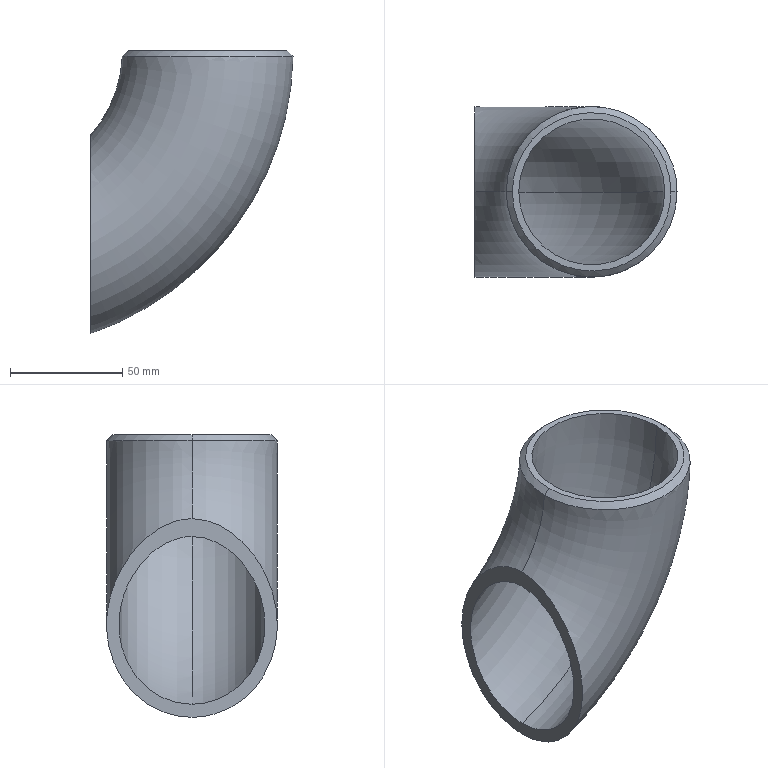Part | SolidWorks | features Chamfer 1, Revolution 1, Split 1 | 1 solid | 8 faces | box 89.972 x 76 x 125.857 mm | volume 125660 mm3 | torus 4 | spline 2 | plane 2
STEP:
#1=CARTESIAN_POINT('',(43.,0.,-37.417));
#2=VERTEX_POINT('',#1);
#3=CARTESIAN_POINT('',(43.,0.,-125.857));
#4=VERTEX_POINT('',#3);
#5=CARTESIAN_POINT('',(43.,0.,-37.417));
#6=CARTESIAN_POINT('',(43.,-2.709,-37.417));
#7=CARTESIAN_POINT('',(43.,-5.352,-37.856));
#8=CARTESIAN_POINT('',(43.,-9.232,-39.095));
#9=CARTESIAN_POINT('',(43.,-10.484,-39.596));
#10=CARTESIAN_POINT('',(43.,-12.905,-40.744));
#11=CARTESIAN_POINT('',(43.,-14.077,-41.391));
#12=CARTESIAN_POINT('',(43.,-15.785,-42.457));
#13=CARTESIAN_POINT('',(43.,-16.345,-42.829));
#14=CARTESIAN_POINT('',(43.,-17.45,-43.603));
#15=CARTESIAN_POINT('',(43.,-17.996,-44.006));
#16=CARTESIAN_POINT('',(43.,-19.594,-45.248));
#17=CARTESIAN_POINT('',(43.,-20.612,-46.122));
#18=CARTESIAN_POINT('',(43.,-23.541,-48.861));
#19=CARTESIAN_POINT('',(43.,-25.328,-50.845));
#20=CARTESIAN_POINT('',(43.,-27.377,-53.503));
#21=CARTESIAN_POINT('',(43.,-27.777,-54.043));
#22=CARTESIAN_POINT('',(43.,-28.559,-55.142));
#23=CARTESIAN_POINT('',(43.,-28.94,-55.7));
#24=CARTESIAN_POINT('',(43.,-30.047,-57.389));
#25=CARTESIAN_POINT('',(43.,-30.74,-58.538));
#26=CARTESIAN_POINT('',(43.,-32.684,-62.049));
#27=CARTESIAN_POINT('',(43.,-33.803,-64.476));
#28=CARTESIAN_POINT('',(43.,-34.976,-67.621));
#29=CARTESIAN_POINT('',(43.,-35.199,-68.256));
#30=CARTESIAN_POINT('',(43.,-35.622,-69.536));
#31=CARTESIAN_POINT('',(43.,-35.822,-70.182));
#32=CARTESIAN_POINT('',(43.,-36.381,-72.122));
#33=CARTESIAN_POINT('',(43.,-36.702,-73.421));
#34=CARTESIAN_POINT('',(43.,-37.509,-77.339));
#35=CARTESIAN_POINT('',(43.,-37.841,-79.978));
#36=CARTESIAN_POINT('',(43.,-38.013,-83.978));
#37=CARTESIAN_POINT('',(43.,-38.015,-85.318));
#38=CARTESIAN_POINT('',(43.,-37.932,-87.34));
#39=CARTESIAN_POINT('',(43.,-37.89,-88.016));
#40=CARTESIAN_POINT('',(43.,-37.776,-89.358));
#41=CARTESIAN_POINT('',(43.,-37.705,-90.025));
#42=CARTESIAN_POINT('',(43.,-37.277,-93.344));
#43=CARTESIAN_POINT('',(43.,-36.707,-95.942));
#44=CARTESIAN_POINT('',(43.,-35.496,-99.749));
#45=CARTESIAN_POINT('',(43.,-35.033,-101.003));
#46=CARTESIAN_POINT('',(43.,-34.243,-102.861));
#47=CARTESIAN_POINT('',(43.,-33.963,-103.477));
#48=CARTESIAN_POINT('',(43.,-33.374,-104.695));
#49=CARTESIAN_POINT('',(43.,-33.066,-105.295));
#50=CARTESIAN_POINT('',(43.,-31.456,-108.246));
#51=CARTESIAN_POINT('',(43.,-29.95,-110.458));
#52=CARTESIAN_POINT('',(43.,-27.786,-113.027));
#53=CARTESIAN_POINT('',(43.,-27.339,-113.531));
#54=CARTESIAN_POINT('',(43.,-26.415,-114.518));
#55=CARTESIAN_POINT('',(43.,-25.939,-115.001));
#56=CARTESIAN_POINT('',(43.,-24.483,-116.403));
#57=CARTESIAN_POINT('',(43.,-23.47,-117.28));
#58=CARTESIAN_POINT('',(43.,-21.36,-118.92));
#59=CARTESIAN_POINT('',(43.,-20.263,-119.684));
#60=CARTESIAN_POINT('',(43.,-18.553,-120.741));
#61=CARTESIAN_POINT('',(43.,-17.972,-121.079));
#62=CARTESIAN_POINT('',(43.,-16.788,-121.725));
#63=CARTESIAN_POINT('',(43.,-16.184,-122.034));
#64=CARTESIAN_POINT('',(43.,-13.137,-123.485));
#65=CARTESIAN_POINT('',(43.,-10.613,-124.361));
#66=CARTESIAN_POINT('',(43.,-7.351,-125.105));
#67=CARTESIAN_POINT('',(43.,-6.693,-125.236));
#68=CARTESIAN_POINT('',(43.,-5.366,-125.461));
#69=CARTESIAN_POINT('',(43.,-4.695,-125.556));
#70=CARTESIAN_POINT('',(43.,-2.678,-125.783));
#71=CARTESIAN_POINT('',(43.,-1.337,-125.857));
#72=CARTESIAN_POINT('',(43.,0.,-125.857));
#73=B_SPLINE_CURVE_WITH_KNOTS('',3,(#5,#6,#7,#8,#9,#10,#11,#12,#13,#14,#15,#16,#17,#18,#19,#20,#21,#22,#23,#24,#25,#26,#27,#28,#29,#30,#31,#32,#33,#34,#35,#36,#37,#38,#39,#40,#41,#42,#43,#44,#45,#46,#47,#48,#49,#50,#51,#52,#53,#54,#55,#56,#57,#58,#59,#60,#61,#62,#63,#64,#65,#66,#67,#68,#69,#70,#71,#72),.UNSPECIFIED.,.F.,.F.,(4,2,2,2,2,2,2,2,2,2,2,2,2,2,2,2,2,2,2,2,2,2,2,2,2,2,2,2,2,2,2,2,2,4),(0.1576,0.1656,0.1696,0.1736,0.1756,0.1776,0.1816,0.1896,0.1916,0.1936,0.1977,0.2057,0.2077,0.2097,0.2137,0.2217,0.2257,0.2277,0.2297,0.2377,0.2417,0.2437,0.2457,0.2538,0.2558,0.2578,0.2618,0.2658,0.2678,0.2698,0.2778,0.2798,0.2818,0.2858),.UNSPECIFIED.);
#74=EDGE_CURVE('',#2,#4,#73,.T.);
#75=ORIENTED_EDGE('',*,*,#74,.T.);
#76=CARTESIAN_POINT('',(132.972,0.,-2.722));
#77=VERTEX_POINT('',#76);
#78=CARTESIAN_POINT('',(0.,0.,0.));
#79=DIRECTION('',(0.,-1.,0.));
#80=DIRECTION('',(0.,0.,-1.));
#81=AXIS2_PLACEMENT_3D('',#78,#79,#80);
#82=CIRCLE('',#81,133.);
#83=EDGE_CURVE('',#4,#77,#82,.T.);
#84=ORIENTED_EDGE('',*,*,#83,.T.);
#85=CARTESIAN_POINT('',(56.943,-0.01359,-2.545));
#86=VERTEX_POINT('',#85);
#87=CARTESIAN_POINT('',(132.972,0.,-2.722));
#88=CARTESIAN_POINT('',(132.972,-2.665,-2.722));
#89=CARTESIAN_POINT('',(132.691,-5.307,-2.722));
#90=CARTESIAN_POINT('',(131.605,-10.435,-2.72));
#91=CARTESIAN_POINT('',(130.801,-12.92,-2.719));
#92=CARTESIAN_POINT('',(128.728,-17.638,-2.717));
#93=CARTESIAN_POINT('',(127.461,-19.87,-2.716));
#94=CARTESIAN_POINT('',(124.537,-24.005,-2.713));
#95=CARTESIAN_POINT('',(122.881,-25.907,-2.711));
#96=CARTESIAN_POINT('',(119.264,-29.325,-2.707));
#97=CARTESIAN_POINT('',(117.304,-30.84,-2.704));
#98=CARTESIAN_POINT('',(113.17,-33.446,-2.699));
#99=CARTESIAN_POINT('',(110.996,-34.537,-2.696));
#100=CARTESIAN_POINT('',(106.524,-36.279,-2.688));
#101=CARTESIAN_POINT('',(104.227,-36.929,-2.684));
#102=CARTESIAN_POINT('',(100.754,-37.575,-2.678));
#103=CARTESIAN_POINT('',(99.592,-37.735,-2.676));
#104=CARTESIAN_POINT('',(97.849,-37.895,-2.672));
#105=CARTESIAN_POINT('',(97.268,-37.934,-2.671));
#106=CARTESIAN_POINT('',(96.399,-37.974,-2.669));
#107=CARTESIAN_POINT('',(96.109,-37.984,-2.669));
#108=CARTESIAN_POINT('',(95.53,-37.997,-2.668));
#109=CARTESIAN_POINT('',(95.242,-38.,-2.667));
#110=CARTESIAN_POINT('',(92.627,-37.999,-2.662));
#111=CARTESIAN_POINT('',(90.221,-37.785,-2.657));
#112=CARTESIAN_POINT('',(86.56,-37.081,-2.648));
#113=CARTESIAN_POINT('',(85.331,-36.782,-2.645));
#114=CARTESIAN_POINT('',(83.487,-36.233,-2.641));
#115=CARTESIAN_POINT('',(82.872,-36.033,-2.639));
#116=CARTESIAN_POINT('',(81.951,-35.706,-2.636));
#117=CARTESIAN_POINT('',(81.49,-35.536,-2.635));
#118=CARTESIAN_POINT('',(80.954,-35.327,-2.634));
#119=CARTESIAN_POINT('',(80.687,-35.219,-2.633));
#120=CARTESIAN_POINT('',(80.553,-35.164,-2.633));
#121=CARTESIAN_POINT('',(80.496,-35.141,-2.633));
#122=CARTESIAN_POINT('',(80.457,-35.125,-2.632));
#123=CARTESIAN_POINT('',(80.437,-35.117,-2.632));
#124=CARTESIAN_POINT('',(78.122,-34.159,-2.626));
#125=CARTESIAN_POINT('',(75.919,-32.982,-2.618));
#126=CARTESIAN_POINT('',(72.818,-30.913,-2.607));
#127=CARTESIAN_POINT('',(71.818,-30.172,-2.604));
#128=CARTESIAN_POINT('',(70.377,-28.99,-2.599));
#129=CARTESIAN_POINT('',(69.906,-28.585,-2.598));
#130=CARTESIAN_POINT('',(69.215,-27.959,-2.596));
#131=CARTESIAN_POINT('',(68.873,-27.642,-2.595));
#132=CARTESIAN_POINT('',(68.481,-27.265,-2.594));
#133=CARTESIAN_POINT('',(68.287,-27.075,-2.594));
#134=CARTESIAN_POINT('',(68.19,-26.979,-2.593));
#135=CARTESIAN_POINT('',(68.142,-26.932,-2.593));
#136=CARTESIAN_POINT('',(68.122,-26.911,-2.593));
#137=CARTESIAN_POINT('',(68.108,-26.897,-2.593));
#138=CARTESIAN_POINT('',(68.102,-26.892,-2.593));
#139=CARTESIAN_POINT('',(66.006,-24.799,-2.589));
#140=CARTESIAN_POINT('',(64.246,-22.556,-2.58));
#141=CARTESIAN_POINT('',(61.346,-17.956,-2.565));
#142=CARTESIAN_POINT('',(60.206,-15.6,-2.558));
#143=CARTESIAN_POINT('',(58.468,-10.938,-2.549));
#144=CARTESIAN_POINT('',(57.869,-8.632,-2.546));
#145=CARTESIAN_POINT('',(57.297,-5.295,-2.545));
#146=CARTESIAN_POINT('',(57.161,-4.203,-2.545));
#147=CARTESIAN_POINT('',(57.029,-2.602,-2.545));
#148=CARTESIAN_POINT('',(56.996,-2.075,-2.545));
#149=CARTESIAN_POINT('',(56.964,-1.294,-2.545));
#150=CARTESIAN_POINT('',(56.952,-0.9063,-2.545));
#151=CARTESIAN_POINT('',(56.946,-0.4584,-2.545));
#152=CARTESIAN_POINT('',(56.944,-0.2356,-2.545));
#153=CARTESIAN_POINT('',(56.943,-0.1245,-2.545));
#154=CARTESIAN_POINT('',(56.943,-0.06902,-2.545));
#155=CARTESIAN_POINT('',(56.943,-0.04526,-2.545));
#156=CARTESIAN_POINT('',(56.943,-0.02942,-2.545));
#157=CARTESIAN_POINT('',(56.943,-0.02269,-2.545));
#158=CARTESIAN_POINT('',(56.943,-0.01359,-2.545));
#159=B_SPLINE_CURVE_WITH_KNOTS('',3,(#87,#88,#89,#90,#91,#92,#93,#94,#95,#96,#97,#98,#99,#100,#101,#102,#103,#104,#105,#106,#107,#108,#109,#110,#111,#112,#113,#114,#115,#116,#117,#118,#119,#120,#121,#122,#123,#124,#125,#126,#127,#128,#129,#130,#131,#132,#133,#134,#135,#136,#137,#138,#139,#140,#141,#142,#143,#144,#145,#146,#147,#148,#149,#150,#151,#152,#153,#154,#155,#156,#157,#158),.UNSPECIFIED.,.F.,.F.,(4,2,2,2,2,2,2,2,2,2,2,2,2,2,2,1,1,1,1,2,2,2,2,2,1,1,1,1,1,2,2,2,2,2,2,2,1,1,1,1,1,2,4),(0.,0.03125,0.0625,0.09375,0.125,0.1563,0.1875,0.2188,0.2344,0.2422,0.2461,0.25,0.2813,0.2969,0.3047,0.3086,0.3105,0.3115,0.312,0.3123,0.3125,0.3438,0.3594,0.3672,0.3711,0.373,0.374,0.3745,0.3748,0.3749,0.375,0.4063,0.4375,0.4688,0.4844,0.4922,0.4961,0.498,0.499,0.4995,0.4998,0.4999,0.5),.UNSPECIFIED.);
#160=EDGE_CURVE('',#77,#86,#159,.T.);
#161=ORIENTED_EDGE('',*,*,#160,.T.);
#162=CARTESIAN_POINT('',(0.,0.,0.));
#163=DIRECTION('',(0.,-1.,0.));
#164=DIRECTION('',(0.,0.,-1.));
#165=AXIS2_PLACEMENT_3D('',#162,#163,#164);
#166=CIRCLE('',#165,57.);
#167=EDGE_CURVE('',#2,#86,#166,.T.);
#168=ORIENTED_EDGE('',*,*,#167,.F.);
#169=EDGE_LOOP('',(#75,#84,#161,#168));
#170=FACE_OUTER_BOUND('',#169,.T.);
#171=CARTESIAN_POINT('',(0.,0.,0.));
#172=DIRECTION('',(0.,-1.,0.));
#173=DIRECTION('',(0.,0.,-1.));
#174=AXIS2_PLACEMENT_3D('',#171,#172,#173);
#175=TOROIDAL_SURFACE('',#174,95.,38.);
#176=ADVANCED_FACE('',(#170),#175,.T.);
#177=CARTESIAN_POINT('',(59.663,-0.01262,0.));
#178=VERTEX_POINT('',#177);
#179=CARTESIAN_POINT('',(130.25,0.,0.));
#180=VERTEX_POINT('',#179);
#181=CARTESIAN_POINT('',(59.663,-0.01262,0.));
#182=CARTESIAN_POINT('',(59.666,-2.359,0.));
#183=CARTESIAN_POINT('',(60.005,-5.807,0.));
#184=CARTESIAN_POINT('',(60.987,-9.705,0.));
#185=CARTESIAN_POINT('',(61.533,-11.349,0.));
#186=CARTESIAN_POINT('',(61.926,-12.44,0.));
#187=CARTESIAN_POINT('',(62.135,-12.98,0.));
#188=CARTESIAN_POINT('',(63.259,-15.684,0.));
#189=CARTESIAN_POINT('',(64.89,-18.736,0.));
#190=CARTESIAN_POINT('',(67.288,-21.959,0.));
#191=CARTESIAN_POINT('',(68.422,-23.268,0.));
#192=CARTESIAN_POINT('',(69.202,-24.125,0.));
#193=CARTESIAN_POINT('',(69.603,-24.544,0.));
#194=CARTESIAN_POINT('',(73.331,-28.262,0.));
#195=CARTESIAN_POINT('',(77.146,-30.808,0.));
#196=CARTESIAN_POINT('',(83.617,-33.486,0.));
#197=CARTESIAN_POINT('',(86.922,-34.491,0.));
#198=CARTESIAN_POINT('',(90.897,-35.079,0.));
#199=CARTESIAN_POINT('',(92.627,-35.206,0.));
#200=CARTESIAN_POINT('',(93.785,-35.262,0.));
#201=CARTESIAN_POINT('',(94.369,-35.277,0.));
#202=CARTESIAN_POINT('',(97.287,-35.279,0.));
#203=CARTESIAN_POINT('',(100.725,-34.946,0.));
#204=CARTESIAN_POINT('',(104.068,-34.108,0.));
#205=CARTESIAN_POINT('',(106.276,-33.437,0.));
#206=CARTESIAN_POINT('',(107.371,-33.045,0.));
#207=CARTESIAN_POINT('',(112.775,-30.812,0.));
#208=CARTESIAN_POINT('',(116.594,-28.263,0.));
#209=CARTESIAN_POINT('',(121.565,-23.297,0.));
#210=CARTESIAN_POINT('',(123.764,-20.624,0.));
#211=CARTESIAN_POINT('',(125.536,-17.666,0.));
#212=CARTESIAN_POINT('',(126.621,-15.63,0.));
#213=CARTESIAN_POINT('',(127.116,-14.582,0.));
#214=CARTESIAN_POINT('',(129.357,-9.17,0.));
#215=CARTESIAN_POINT('',(130.252,-4.67,0.));
#216=CARTESIAN_POINT('',(130.25,0.,0.));
#217=B_SPLINE_CURVE_WITH_KNOTS('',3,(#181,#182,#183,#184,#185,#186,#187,#188,#189,#190,#191,#192,#193,#194,#195,#196,#197,#198,#199,#200,#201,#202,#203,#204,#205,#206,#207,#208,#209,#210,#211,#212,#213,#214,#215,#216),.UNSPECIFIED.,.F.,.F.,(4,1,1,2,2,1,1,2,2,2,1,1,2,2,1,2,2,2,1,2,2,4),(0.5,0.5312,0.5469,0.5547,0.5625,0.5938,0.6094,0.6172,0.625,0.6875,0.7187,0.7344,0.7422,0.75,0.7812,0.7969,0.8125,0.875,0.9062,0.9219,0.9375,1.),.UNSPECIFIED.);
#218=EDGE_CURVE('',#178,#180,#217,.T.);
#219=ORIENTED_EDGE('',*,*,#218,.F.);
#220=CARTESIAN_POINT('',(59.663,-0.01262,0.));
#221=CARTESIAN_POINT('',(56.943,-0.01359,-2.545));
#222=B_SPLINE_CURVE_WITH_KNOTS('',1,(#220,#221),.UNSPECIFIED.,.F.,.F.,(2,2),(0.,1.),.UNSPECIFIED.);
#223=EDGE_CURVE('',#178,#86,#222,.T.);
#224=ORIENTED_EDGE('',*,*,#223,.T.);
#225=ORIENTED_EDGE('',*,*,#160,.F.);
#226=CARTESIAN_POINT('',(130.25,0.,0.));
#227=CARTESIAN_POINT('',(132.972,0.,-2.722));
#228=B_SPLINE_CURVE_WITH_KNOTS('',1,(#226,#227),.UNSPECIFIED.,.F.,.F.,(2,2),(0.,1.),.UNSPECIFIED.);
#229=EDGE_CURVE('',#180,#77,#228,.T.);
#230=ORIENTED_EDGE('',*,*,#229,.F.);
#231=EDGE_LOOP('',(#219,#224,#225,#230));
#232=FACE_OUTER_BOUND('',#231,.T.);
#233=CARTESIAN_POINT('',(130.25,0.,0.));
#234=CARTESIAN_POINT('',(130.249,2.299,0.));
#235=CARTESIAN_POINT('',(130.028,4.585,0.));
#236=CARTESIAN_POINT('',(129.123,9.145,0.));
#237=CARTESIAN_POINT('',(128.445,11.372,0.));
#238=CARTESIAN_POINT('',(126.689,15.614,0.));
#239=CARTESIAN_POINT('',(125.599,17.66,0.));
#240=CARTESIAN_POINT('',(123.011,21.532,0.));
#241=CARTESIAN_POINT('',(121.549,23.308,0.));
#242=CARTESIAN_POINT('',(118.305,26.558,0.));
#243=CARTESIAN_POINT('',(116.488,28.051,0.));
#244=CARTESIAN_POINT('',(112.647,30.614,0.));
#245=CARTESIAN_POINT('',(110.623,31.697,0.));
#246=CARTESIAN_POINT('',(106.353,33.47,0.));
#247=CARTESIAN_POINT('',(104.106,34.151,0.));
#248=CARTESIAN_POINT('',(99.603,35.045,0.));
#249=CARTESIAN_POINT('',(97.312,35.276,0.));
#250=CARTESIAN_POINT('',(92.651,35.279,0.));
#251=CARTESIAN_POINT('',(90.35,35.049,0.));
#252=CARTESIAN_POINT('',(85.847,34.158,0.));
#253=CARTESIAN_POINT('',(83.612,33.484,0.));
#254=CARTESIAN_POINT('',(79.323,31.709,0.));
#255=CARTESIAN_POINT('',(77.298,30.626,0.));
#256=CARTESIAN_POINT('',(73.467,28.076,0.));
#257=CARTESIAN_POINT('',(71.644,26.583,0.));
#258=CARTESIAN_POINT('',(68.39,23.331,0.));
#259=CARTESIAN_POINT('',(66.928,21.56,0.));
#260=CARTESIAN_POINT('',(64.342,17.702,0.));
#261=CARTESIAN_POINT('',(63.242,15.645,0.));
#262=CARTESIAN_POINT('',(60.602,9.288,0.));
#263=CARTESIAN_POINT('',(59.658,4.638,0.));
#264=CARTESIAN_POINT('',(59.666,-2.338,0.));
#265=CARTESIAN_POINT('',(59.895,-4.639,0.));
#266=CARTESIAN_POINT('',(60.791,-9.141,0.));
#267=CARTESIAN_POINT('',(61.471,-11.382,0.));
#268=CARTESIAN_POINT('',(63.249,-15.66,0.));
#269=CARTESIAN_POINT('',(64.334,-17.683,0.));
#270=CARTESIAN_POINT('',(66.895,-21.516,0.));
#271=CARTESIAN_POINT('',(68.39,-23.335,0.));
#272=CARTESIAN_POINT('',(71.644,-26.58,0.));
#273=CARTESIAN_POINT('',(73.419,-28.04,0.));
#274=CARTESIAN_POINT('',(77.288,-30.624,0.));
#275=CARTESIAN_POINT('',(79.339,-31.716,0.));
#276=CARTESIAN_POINT('',(83.581,-33.471,0.));
#277=CARTESIAN_POINT('',(85.802,-34.148,0.));
#278=CARTESIAN_POINT('',(90.368,-35.054,0.));
#279=CARTESIAN_POINT('',(92.656,-35.276,0.));
#280=CARTESIAN_POINT('',(97.25,-35.279,0.));
#281=CARTESIAN_POINT('',(99.592,-35.049,0.));
#282=CARTESIAN_POINT('',(104.115,-34.147,0.));
#283=CARTESIAN_POINT('',(106.313,-33.482,0.));
#284=CARTESIAN_POINT('',(110.591,-31.715,0.));
#285=CARTESIAN_POINT('',(112.658,-30.609,0.));
#286=CARTESIAN_POINT('',(116.474,-28.058,0.));
#287=CARTESIAN_POINT('',(118.259,-26.6,0.));
#288=CARTESIAN_POINT('',(121.557,-23.305,0.));
#289=CARTESIAN_POINT('',(123.02,-21.517,0.));
#290=CARTESIAN_POINT('',(125.573,-17.702,0.));
#291=CARTESIAN_POINT('',(126.677,-15.642,0.));
#292=CARTESIAN_POINT('',(128.452,-11.357,0.));
#293=CARTESIAN_POINT('',(129.117,-9.159,0.));
#294=CARTESIAN_POINT('',(130.02,-4.643,0.));
#295=CARTESIAN_POINT('',(130.251,-2.299,0.));
#296=CARTESIAN_POINT('',(130.25,0.,0.));
#297=CARTESIAN_POINT('',(132.972,0.,-2.722));
#298=CARTESIAN_POINT('',(132.971,2.476,-2.722));
#299=CARTESIAN_POINT('',(132.733,4.939,-2.722));
#300=CARTESIAN_POINT('',(131.758,9.851,-2.721));
#301=CARTESIAN_POINT('',(131.028,12.25,-2.72));
#302=CARTESIAN_POINT('',(129.136,16.819,-2.718));
#303=CARTESIAN_POINT('',(127.963,19.023,-2.717));
#304=CARTESIAN_POINT('',(125.175,23.194,-2.713));
#305=CARTESIAN_POINT('',(123.6,25.107,-2.711));
#306=CARTESIAN_POINT('',(120.105,28.608,-2.707));
#307=CARTESIAN_POINT('',(118.148,30.216,-2.704));
#308=CARTESIAN_POINT('',(114.011,32.977,-2.699));
#309=CARTESIAN_POINT('',(111.831,34.143,-2.696));
#310=CARTESIAN_POINT('',(107.231,36.053,-2.689));
#311=CARTESIAN_POINT('',(104.811,36.787,-2.685));
#312=CARTESIAN_POINT('',(99.961,37.75,-2.676));
#313=CARTESIAN_POINT('',(97.493,37.999,-2.671));
#314=CARTESIAN_POINT('',(92.473,38.001,-2.661));
#315=CARTESIAN_POINT('',(89.994,37.754,-2.656));
#316=CARTESIAN_POINT('',(85.144,36.794,-2.645));
#317=CARTESIAN_POINT('',(82.737,36.068,-2.639));
#318=CARTESIAN_POINT('',(78.117,34.156,-2.626));
#319=CARTESIAN_POINT('',(75.936,32.99,-2.62));
#320=CARTESIAN_POINT('',(71.81,30.243,-2.606));
#321=CARTESIAN_POINT('',(69.846,28.635,-2.6));
#322=CARTESIAN_POINT('',(66.341,25.132,-2.587));
#323=CARTESIAN_POINT('',(64.768,23.224,-2.58));
#324=CARTESIAN_POINT('',(61.982,19.069,-2.569));
#325=CARTESIAN_POINT('',(60.797,16.852,-2.563));
#326=CARTESIAN_POINT('',(57.954,10.005,-2.55));
#327=CARTESIAN_POINT('',(56.938,4.996,-2.545));
#328=CARTESIAN_POINT('',(56.946,-2.518,-2.545));
#329=CARTESIAN_POINT('',(57.193,-4.997,-2.546));
#330=CARTESIAN_POINT('',(58.158,-9.847,-2.551));
#331=CARTESIAN_POINT('',(58.89,-12.261,-2.555));
#332=CARTESIAN_POINT('',(60.805,-16.869,-2.563));
#333=CARTESIAN_POINT('',(61.973,-19.048,-2.569));
#334=CARTESIAN_POINT('',(64.731,-23.177,-2.58));
#335=CARTESIAN_POINT('',(66.342,-25.136,-2.587));
#336=CARTESIAN_POINT('',(69.846,-28.631,-2.6));
#337=CARTESIAN_POINT('',(71.758,-30.204,-2.606));
#338=CARTESIAN_POINT('',(75.925,-32.987,-2.62));
#339=CARTESIAN_POINT('',(78.135,-34.164,-2.626));
#340=CARTESIAN_POINT('',(82.703,-36.055,-2.639));
#341=CARTESIAN_POINT('',(85.096,-36.783,-2.645));
#342=CARTESIAN_POINT('',(90.013,-37.76,-2.656));
#343=CARTESIAN_POINT('',(92.478,-37.998,-2.661));
#344=CARTESIAN_POINT('',(97.426,-38.002,-2.671));
#345=CARTESIAN_POINT('',(99.949,-37.754,-2.676));
#346=CARTESIAN_POINT('',(104.821,-36.783,-2.685));
#347=CARTESIAN_POINT('',(107.188,-36.066,-2.688));
#348=CARTESIAN_POINT('',(111.796,-34.162,-2.696));
#349=CARTESIAN_POINT('',(114.023,-32.971,-2.699));
#350=CARTESIAN_POINT('',(118.133,-30.223,-2.704));
#351=CARTESIAN_POINT('',(120.056,-28.653,-2.707));
#352=CARTESIAN_POINT('',(123.608,-25.103,-2.711));
#353=CARTESIAN_POINT('',(125.184,-23.178,-2.713));
#354=CARTESIAN_POINT('',(127.934,-19.068,-2.717));
#355=CARTESIAN_POINT('',(129.124,-16.849,-2.718));
#356=CARTESIAN_POINT('',(131.035,-12.233,-2.72));
#357=CARTESIAN_POINT('',(131.751,-9.866,-2.721));
#358=CARTESIAN_POINT('',(132.724,-5.002,-2.722));
#359=CARTESIAN_POINT('',(132.973,-2.476,-2.722));
#360=CARTESIAN_POINT('',(132.972,0.,-2.722));
#361=B_SPLINE_SURFACE_WITH_KNOTS('',1,3,((#233,#234,#235,#236,#237,#238,#239,#240,#241,#242,#243,#244,#245,#246,#247,#248,#249,#250,#251,#252,#253,#254,#255,#256,#257,#258,#259,#260,#261,#262,#263,#264,#265,#266,#267,#268,#269,#270,#271,#272,#273,#274,#275,#276,#277,#278,#279,#280,#281,#282,#283,#284,#285,#286,#287,#288,#289,#290,#291,#292,#293,#294,#295,#296),(#297,#298,#299,#300,#301,#302,#303,#304,#305,#306,#307,#308,#309,#310,#311,#312,#313,#314,#315,#316,#317,#318,#319,#320,#321,#322,#323,#324,#325,#326,#327,#328,#329,#330,#331,#332,#333,#334,#335,#336,#337,#338,#339,#340,#341,#342,#343,#344,#345,#346,#347,#348,#349,#350,#351,#352,#353,#354,#355,#356,#357,#358,#359,#360)),.UNSPECIFIED.,.F.,.T.,.F.,(2,2),(4,2,2,2,2,2,2,2,2,2,2,2,2,2,2,2,2,2,2,2,2,2,2,2,2,2,2,2,2,2,2,4),(0.,1.),(0.00369,0.01058,0.01748,0.02437,0.03127,0.03816,0.04505,0.05195,0.05884,0.06574,0.07263,0.07952,0.08642,0.09331,0.1002,0.114,0.1209,0.1278,0.1347,0.1416,0.1485,0.1554,0.1623,0.1691,0.176,0.1829,0.1898,0.1967,0.2036,0.2105,0.2174,0.2243),.UNSPECIFIED.);
#362=ADVANCED_FACE('',(#232),#361,.T.);
#363=CARTESIAN_POINT('',(43.,0.,-120.03));
#364=VERTEX_POINT('',#363);
#365=CARTESIAN_POINT('',(43.,0.,-45.357));
#366=VERTEX_POINT('',#365);
#367=CARTESIAN_POINT('',(43.,0.,-120.03));
#368=CARTESIAN_POINT('',(43.,1.143,-120.03));
#369=CARTESIAN_POINT('',(43.,2.299,-119.965));
#370=CARTESIAN_POINT('',(43.,4.57,-119.709));
#371=CARTESIAN_POINT('',(43.,5.692,-119.518));
#372=CARTESIAN_POINT('',(43.,7.907,-119.014));
#373=CARTESIAN_POINT('',(43.,9.,-118.701));
#374=CARTESIAN_POINT('',(43.,11.159,-117.952));
#375=CARTESIAN_POINT('',(43.,12.23,-117.512));
#376=CARTESIAN_POINT('',(43.,15.327,-116.038));
#377=CARTESIAN_POINT('',(43.,17.26,-114.843));
#378=CARTESIAN_POINT('',(43.,19.97,-112.744));
#379=CARTESIAN_POINT('',(43.,20.845,-111.988));
#380=CARTESIAN_POINT('',(43.,22.496,-110.404));
#381=CARTESIAN_POINT('',(43.,23.275,-109.574));
#382=CARTESIAN_POINT('',(43.,24.746,-107.841));
#383=CARTESIAN_POINT('',(43.,25.437,-106.937));
#384=CARTESIAN_POINT('',(43.,26.408,-105.527));
#385=CARTESIAN_POINT('',(43.,26.721,-105.048));
#386=CARTESIAN_POINT('',(43.,27.324,-104.072));
#387=CARTESIAN_POINT('',(43.,27.615,-103.575));
#388=CARTESIAN_POINT('',(43.,28.999,-101.067));
#389=CARTESIAN_POINT('',(43.,29.899,-98.979));
#390=CARTESIAN_POINT('',(43.,30.959,-95.732));
#391=CARTESIAN_POINT('',(43.,31.264,-94.63));
#392=CARTESIAN_POINT('',(43.,31.776,-92.388));
#393=CARTESIAN_POINT('',(43.,31.979,-91.263));
#394=CARTESIAN_POINT('',(43.,32.442,-87.879));
#395=CARTESIAN_POINT('',(43.,32.554,-85.609));
#396=CARTESIAN_POINT('',(43.,32.438,-82.185));
#397=CARTESIAN_POINT('',(43.,32.351,-81.036));
#398=CARTESIAN_POINT('',(43.,32.087,-78.764));
#399=CARTESIAN_POINT('',(43.,31.909,-77.639));
#400=CARTESIAN_POINT('',(43.,31.245,-74.296));
#401=CARTESIAN_POINT('',(43.,30.628,-72.11));
#402=CARTESIAN_POINT('',(43.,29.446,-68.894));
#403=CARTESIAN_POINT('',(43.,29.007,-67.829));
#404=CARTESIAN_POINT('',(43.,28.054,-65.752));
#405=CARTESIAN_POINT('',(43.,27.54,-64.738));
#406=CARTESIAN_POINT('',(43.,25.887,-61.764));
#407=CARTESIAN_POINT('',(43.,24.636,-59.875));
#408=CARTESIAN_POINT('',(43.,22.876,-57.637));
#409=CARTESIAN_POINT('',(43.,22.514,-57.196));
#410=CARTESIAN_POINT('',(43.,21.77,-56.326));
#411=CARTESIAN_POINT('',(43.,21.386,-55.897));
#412=CARTESIAN_POINT('',(43.,20.212,-54.64));
#413=CARTESIAN_POINT('',(43.,19.397,-53.841));
#414=CARTESIAN_POINT('',(43.,16.854,-51.566));
#415=CARTESIAN_POINT('',(43.,15.028,-50.21));
#416=CARTESIAN_POINT('',(43.,12.544,-48.763));
#417=CARTESIAN_POINT('',(43.,12.038,-48.486));
#418=CARTESIAN_POINT('',(43.,11.017,-47.967));
#419=CARTESIAN_POINT('',(43.,10.5,-47.724));
#420=CARTESIAN_POINT('',(43.,8.933,-47.042));
#421=CARTESIAN_POINT('',(43.,7.863,-46.652));
#422=CARTESIAN_POINT('',(43.,6.219,-46.174));
#423=CARTESIAN_POINT('',(43.,5.665,-46.033));
#424=CARTESIAN_POINT('',(43.,4.541,-45.789));
#425=CARTESIAN_POINT('',(43.,3.972,-45.685));
#426=CARTESIAN_POINT('',(43.,2.27,-45.439));
#427=CARTESIAN_POINT('',(43.,1.135,-45.357));
#428=CARTESIAN_POINT('',(43.,0.,-45.357));
#429=B_SPLINE_CURVE_WITH_KNOTS('',3,(#367,#368,#369,#370,#371,#372,#373,#374,#375,#376,#377,#378,#379,#380,#381,#382,#383,#384,#385,#386,#387,#388,#389,#390,#391,#392,#393,#394,#395,#396,#397,#398,#399,#400,#401,#402,#403,#404,#405,#406,#407,#408,#409,#410,#411,#412,#413,#414,#415,#416,#417,#418,#419,#420,#421,#422,#423,#424,#425,#426,#427,#428),.UNSPECIFIED.,.F.,.F.,(4,2,2,2,2,2,2,2,2,2,2,2,2,2,2,2,2,2,2,2,2,2,2,2,2,2,2,2,2,2,4),(0.01925,0.02266,0.02607,0.02948,0.03288,0.0397,0.0431,0.04651,0.04992,0.05162,0.05333,0.06014,0.06355,0.06695,0.07377,0.07718,0.08058,0.0874,0.09081,0.09421,0.101,0.1027,0.1044,0.1078,0.1147,0.1164,0.1181,0.1215,0.1232,0.1249,0.1283),.UNSPECIFIED.);
#430=EDGE_CURVE('',#364,#366,#429,.T.);
#431=ORIENTED_EDGE('',*,*,#430,.F.);
#432=CARTESIAN_POINT('',(127.5,0.,0.));
#433=VERTEX_POINT('',#432);
#434=CARTESIAN_POINT('',(0.,0.,0.));
#435=DIRECTION('',(0.,-1.,0.));
#436=DIRECTION('',(0.,0.,-1.));
#437=AXIS2_PLACEMENT_3D('',#434,#435,#436);
#438=CIRCLE('',#437,127.5);
#439=EDGE_CURVE('',#364,#433,#438,.T.);
#440=ORIENTED_EDGE('',*,*,#439,.T.);
#441=CARTESIAN_POINT('',(62.5,0.,0.));
#442=VERTEX_POINT('',#441);
#443=CARTESIAN_POINT('',(95.,0.,0.));
#444=DIRECTION('',(0.,0.,1.));
#445=DIRECTION('',(1.,0.,0.));
#446=AXIS2_PLACEMENT_3D('',#443,#444,#445);
#447=CIRCLE('',#446,32.5);
#448=EDGE_CURVE('',#433,#442,#447,.T.);
#449=ORIENTED_EDGE('',*,*,#448,.T.);
#450=CARTESIAN_POINT('',(0.,0.,0.));
#451=DIRECTION('',(0.,-1.,0.));
#452=DIRECTION('',(0.,0.,-1.));
#453=AXIS2_PLACEMENT_3D('',#450,#451,#452);
#454=CIRCLE('',#453,62.5);
#455=EDGE_CURVE('',#366,#442,#454,.T.);
#456=ORIENTED_EDGE('',*,*,#455,.F.);
#457=EDGE_LOOP('',(#431,#440,#449,#456));
#458=FACE_OUTER_BOUND('',#457,.T.);
#459=CARTESIAN_POINT('',(0.,0.,0.));
#460=DIRECTION('',(0.,-1.,0.));
#461=DIRECTION('',(0.,0.,-1.));
#462=AXIS2_PLACEMENT_3D('',#459,#460,#461);
#463=TOROIDAL_SURFACE('',#462,95.,32.5);
#464=ADVANCED_FACE('',(#458),#463,.F.);
#465=CARTESIAN_POINT('',(130.25,0.,0.));
#466=CARTESIAN_POINT('',(130.248,4.683,0.));
#467=CARTESIAN_POINT('',(129.354,9.178,0.));
#468=CARTESIAN_POINT('',(126.673,15.651,0.));
#469=CARTESIAN_POINT('',(125.048,18.699,0.));
#470=CARTESIAN_POINT('',(122.654,21.926,0.));
#471=CARTESIAN_POINT('',(121.521,23.238,0.));
#472=CARTESIAN_POINT('',(120.742,24.097,0.));
#473=CARTESIAN_POINT('',(120.339,24.52,0.));
#474=CARTESIAN_POINT('',(118.278,26.584,0.));
#475=CARTESIAN_POINT('',(115.612,28.779,0.));
#476=CARTESIAN_POINT('',(112.163,30.846,0.));
#477=CARTESIAN_POINT('',(110.612,31.626,0.));
#478=CARTESIAN_POINT('',(109.562,32.122,0.));
#479=CARTESIAN_POINT('',(109.028,32.359,0.));
#480=CARTESIAN_POINT('',(104.169,34.377,0.));
#481=CARTESIAN_POINT('',(99.665,35.275,0.));
#482=CARTESIAN_POINT('',(92.64,35.279,0.));
#483=CARTESIAN_POINT('',(90.343,35.056,0.));
#484=CARTESIAN_POINT('',(85.838,34.162,0.));
#485=CARTESIAN_POINT('',(83.632,33.492,0.));
#486=CARTESIAN_POINT('',(79.303,31.701,0.));
#487=CARTESIAN_POINT('',(76.248,30.074,0.));
#488=CARTESIAN_POINT('',(73.02,27.681,0.));
#489=CARTESIAN_POINT('',(71.709,26.549,0.));
#490=CARTESIAN_POINT('',(70.851,25.771,0.));
#491=CARTESIAN_POINT('',(70.431,25.371,0.));
#492=CARTESIAN_POINT('',(68.361,23.302,0.));
#493=CARTESIAN_POINT('',(66.162,20.632,0.));
#494=CARTESIAN_POINT('',(64.095,17.189,0.));
#495=CARTESIAN_POINT('',(63.187,15.385,0.));
#496=CARTESIAN_POINT('',(62.764,14.462,0.));
#497=CARTESIAN_POINT('',(62.589,14.062,0.));
#498=CARTESIAN_POINT('',(62.474,13.795,0.));
#499=CARTESIAN_POINT('',(62.417,13.659,0.));
#500=CARTESIAN_POINT('',(61.92,12.462,0.));
#501=CARTESIAN_POINT('',(61.337,10.837,0.));
#502=CARTESIAN_POINT('',(60.797,8.891,0.));
#503=CARTESIAN_POINT('',(60.562,7.906,0.));
#504=CARTESIAN_POINT('',(60.469,7.481,0.));
#505=CARTESIAN_POINT('',(60.408,7.196,0.));
#506=CARTESIAN_POINT('',(60.379,7.055,0.));
#507=CARTESIAN_POINT('',(60.12,5.761,0.));
#508=CARTESIAN_POINT('',(59.861,4.033,0.));
#509=CARTESIAN_POINT('',(59.712,2.012,0.));
#510=CARTESIAN_POINT('',(59.675,1.,0.));
#511=CARTESIAN_POINT('',(59.667,0.5662,0.));
#512=CARTESIAN_POINT('',(59.664,0.2768,0.));
#513=CARTESIAN_POINT('',(59.663,0.134,0.));
#514=CARTESIAN_POINT('',(59.663,-0.01262,0.));
#515=B_SPLINE_CURVE_WITH_KNOTS('',3,(#465,#466,#467,#468,#469,#470,#471,#472,#473,#474,#475,#476,#477,#478,#479,#480,#481,#482,#483,#484,#485,#486,#487,#488,#489,#490,#491,#492,#493,#494,#495,#496,#497,#498,#499,#500,#501,#502,#503,#504,#505,#506,#507,#508,#509,#510,#511,#512,#513,#514),.UNSPECIFIED.,.F.,.F.,(4,2,1,1,2,2,1,1,2,2,2,2,2,1,1,2,2,1,1,1,1,2,2,1,1,1,2,2,1,1,1,2,4),(0.,0.0625,0.09375,0.1094,0.1172,0.125,0.1562,0.1719,0.1797,0.1875,0.25,0.2812,0.3125,0.3437,0.3594,0.3672,0.375,0.4062,0.4219,0.4297,0.4336,0.4355,0.4375,0.4531,0.4609,0.4648,0.4668,0.4687,0.4844,0.4922,0.4961,0.498,0.5),.UNSPECIFIED.);
#516=EDGE_CURVE('',#180,#178,#515,.T.);
#517=ORIENTED_EDGE('',*,*,#516,.T.);
#518=ORIENTED_EDGE('',*,*,#218,.T.);
#519=EDGE_LOOP('',(#517,#518));
#520=FACE_OUTER_BOUND('',#519,.T.);
#521=CARTESIAN_POINT('',(95.,0.,0.));
#522=DIRECTION('',(0.,0.,1.));
#523=DIRECTION('',(1.,0.,0.));
#524=AXIS2_PLACEMENT_3D('',#521,#522,#523);
#525=CIRCLE('',#524,32.5);
#526=EDGE_CURVE('',#442,#433,#525,.T.);
#527=ORIENTED_EDGE('',*,*,#526,.F.);
#528=ORIENTED_EDGE('',*,*,#448,.F.);
#529=EDGE_LOOP('',(#527,#528));
#530=FACE_BOUND('',#529,.T.);
#531=CARTESIAN_POINT('',(95.,0.,0.));
#532=DIRECTION('',(0.,0.,1.));
#533=DIRECTION('',(1.,0.,0.));
#534=AXIS2_PLACEMENT_3D('',#531,#532,#533);
#535=PLANE('',#534);
#536=ADVANCED_FACE('',(#520,#530),#535,.T.);
#537=ORIENTED_EDGE('',*,*,#439,.F.);
#538=CARTESIAN_POINT('',(43.,0.,-45.357));
#539=CARTESIAN_POINT('',(43.,-1.135,-45.357));
#540=CARTESIAN_POINT('',(43.,-2.271,-45.439));
#541=CARTESIAN_POINT('',(43.,-3.974,-45.685));
#542=CARTESIAN_POINT('',(43.,-4.544,-45.789));
#543=CARTESIAN_POINT('',(43.,-5.668,-46.034));
#544=CARTESIAN_POINT('',(43.,-6.224,-46.176));
#545=CARTESIAN_POINT('',(43.,-7.871,-46.655));
#546=CARTESIAN_POINT('',(43.,-8.944,-47.046));
#547=CARTESIAN_POINT('',(43.,-10.518,-47.732));
#548=CARTESIAN_POINT('',(43.,-11.036,-47.977));
#549=CARTESIAN_POINT('',(43.,-12.062,-48.499));
#550=CARTESIAN_POINT('',(43.,-12.569,-48.776));
#551=CARTESIAN_POINT('',(43.,-15.044,-50.221));
#552=CARTESIAN_POINT('',(43.,-16.87,-51.578));
#553=CARTESIAN_POINT('',(43.,-19.416,-53.859));
#554=CARTESIAN_POINT('',(43.,-20.234,-54.662));
#555=CARTESIAN_POINT('',(43.,-21.803,-56.345));
#556=CARTESIAN_POINT('',(43.,-22.544,-57.214));
#557=CARTESIAN_POINT('',(43.,-24.653,-59.899));
#558=CARTESIAN_POINT('',(43.,-25.904,-61.791));
#559=CARTESIAN_POINT('',(43.,-27.56,-64.775));
#560=CARTESIAN_POINT('',(43.,-28.075,-65.794));
#561=CARTESIAN_POINT('',(43.,-28.791,-67.36));
#562=CARTESIAN_POINT('',(43.,-29.02,-67.888));
#563=CARTESIAN_POINT('',(43.,-29.455,-68.946));
#564=CARTESIAN_POINT('',(43.,-29.662,-69.478));
#565=CARTESIAN_POINT('',(43.,-30.641,-72.153));
#566=CARTESIAN_POINT('',(43.,-31.255,-74.337));
#567=CARTESIAN_POINT('',(43.,-31.916,-77.682));
#568=CARTESIAN_POINT('',(43.,-32.093,-78.808));
#569=CARTESIAN_POINT('',(43.,-32.29,-80.516));
#570=CARTESIAN_POINT('',(43.,-32.345,-81.089));
#571=CARTESIAN_POINT('',(43.,-32.429,-82.233));
#572=CARTESIAN_POINT('',(43.,-32.46,-82.804));
#573=CARTESIAN_POINT('',(43.,-32.552,-85.652));
#574=CARTESIAN_POINT('',(43.,-32.439,-87.914));
#575=CARTESIAN_POINT('',(43.,-31.976,-91.28));
#576=CARTESIAN_POINT('',(43.,-31.774,-92.397));
#577=CARTESIAN_POINT('',(43.,-31.392,-94.066));
#578=CARTESIAN_POINT('',(43.,-31.253,-94.621));
#579=CARTESIAN_POINT('',(43.,-30.946,-95.729));
#580=CARTESIAN_POINT('',(43.,-30.78,-96.281));
#581=CARTESIAN_POINT('',(43.,-29.891,-99.001));
#582=CARTESIAN_POINT('',(43.,-28.99,-101.082));
#583=CARTESIAN_POINT('',(43.,-27.349,-104.057));
#584=CARTESIAN_POINT('',(43.,-26.753,-105.024));
#585=CARTESIAN_POINT('',(43.,-25.459,-106.908));
#586=CARTESIAN_POINT('',(43.,-24.756,-107.828));
#587=CARTESIAN_POINT('',(43.,-22.532,-110.452));
#588=CARTESIAN_POINT('',(43.,-20.886,-112.033));
#589=CARTESIAN_POINT('',(43.,-18.618,-113.791));
#590=CARTESIAN_POINT('',(43.,-18.152,-114.133));
#591=CARTESIAN_POINT('',(43.,-17.207,-114.787));
#592=CARTESIAN_POINT('',(43.,-16.728,-115.1));
#593=CARTESIAN_POINT('',(43.,-15.27,-115.998));
#594=CARTESIAN_POINT('',(43.,-14.27,-116.541));
#595=CARTESIAN_POINT('',(43.,-12.217,-117.517));
#596=CARTESIAN_POINT('',(43.,-11.164,-117.95));
#597=CARTESIAN_POINT('',(43.,-9.541,-118.513));
#598=CARTESIAN_POINT('',(43.,-8.992,-118.687));
#599=CARTESIAN_POINT('',(43.,-7.886,-119.004));
#600=CARTESIAN_POINT('',(43.,-7.33,-119.146));
#601=CARTESIAN_POINT('',(43.,-4.545,-119.777));
#602=CARTESIAN_POINT('',(43.,-2.287,-120.03));
#603=CARTESIAN_POINT('',(43.,0.,-120.03));
#604=B_SPLINE_CURVE_WITH_KNOTS('',3,(#538,#539,#540,#541,#542,#543,#544,#545,#546,#547,#548,#549,#550,#551,#552,#553,#554,#555,#556,#557,#558,#559,#560,#561,#562,#563,#564,#565,#566,#567,#568,#569,#570,#571,#572,#573,#574,#575,#576,#577,#578,#579,#580,#581,#582,#583,#584,#585,#586,#587,#588,#589,#590,#591,#592,#593,#594,#595,#596,#597,#598,#599,#600,#601,#602,#603),.UNSPECIFIED.,.F.,.F.,(4,2,2,2,2,2,2,2,2,2,2,2,2,2,2,2,2,2,2,2,2,2,2,2,2,2,2,2,2,2,2,2,4),(0.1283,0.1317,0.1334,0.1351,0.1385,0.1402,0.1419,0.1487,0.1522,0.1556,0.1624,0.1658,0.1675,0.1692,0.176,0.1794,0.1811,0.1828,0.1897,0.1931,0.1948,0.1965,0.2033,0.2067,0.2101,0.2169,0.2186,0.2203,0.2237,0.2272,0.2289,0.2306,0.2374),.UNSPECIFIED.);
#605=EDGE_CURVE('',#366,#364,#604,.T.);
#606=ORIENTED_EDGE('',*,*,#605,.F.);
#607=ORIENTED_EDGE('',*,*,#455,.T.);
#608=ORIENTED_EDGE('',*,*,#526,.T.);
#609=EDGE_LOOP('',(#537,#606,#607,#608));
#610=FACE_OUTER_BOUND('',#609,.T.);
#611=CARTESIAN_POINT('',(0.,0.,0.));
#612=DIRECTION('',(0.,-1.,0.));
#613=DIRECTION('',(0.,0.,-1.));
#614=AXIS2_PLACEMENT_3D('',#611,#612,#613);
#615=TOROIDAL_SURFACE('',#614,95.,32.5);
#616=ADVANCED_FACE('',(#610),#615,.F.);
#617=ORIENTED_EDGE('',*,*,#223,.F.);
#618=ORIENTED_EDGE('',*,*,#516,.F.);
#619=ORIENTED_EDGE('',*,*,#229,.T.);
#620=CARTESIAN_POINT('',(56.943,-0.01359,-2.545));
#621=CARTESIAN_POINT('',(56.943,0.132,-2.545));
#622=CARTESIAN_POINT('',(56.944,0.28,-2.545));
#623=CARTESIAN_POINT('',(56.947,0.5737,-2.545));
#624=CARTESIAN_POINT('',(56.955,1.015,-2.545));
#625=CARTESIAN_POINT('',(56.97,1.459,-2.545));
#626=CARTESIAN_POINT('',(57.011,2.35,-2.545));
#627=CARTESIAN_POINT('',(57.053,2.949,-2.545));
#628=CARTESIAN_POINT('',(57.223,4.754,-2.546));
#629=CARTESIAN_POINT('',(57.395,5.971,-2.547));
#630=CARTESIAN_POINT('',(58.104,9.644,-2.55));
#631=CARTESIAN_POINT('',(58.833,12.124,-2.554));
#632=CARTESIAN_POINT('',(59.857,14.588,-2.559));
#633=CARTESIAN_POINT('',(59.862,14.6,-2.559));
#634=CARTESIAN_POINT('',(59.874,14.628,-2.559));
#635=CARTESIAN_POINT('',(59.891,14.67,-2.559));
#636=CARTESIAN_POINT('',(59.932,14.767,-2.559));
#637=CARTESIAN_POINT('',(60.015,14.964,-2.56));
#638=CARTESIAN_POINT('',(60.187,15.36,-2.561));
#639=CARTESIAN_POINT('',(60.343,15.707,-2.561));
#640=CARTESIAN_POINT('',(60.668,16.41,-2.563));
#641=CARTESIAN_POINT('',(60.901,16.89,-2.564));
#642=CARTESIAN_POINT('',(61.658,18.36,-2.567));
#643=CARTESIAN_POINT('',(62.237,19.38,-2.569));
#644=CARTESIAN_POINT('',(63.573,21.475,-2.575));
#645=CARTESIAN_POINT('',(64.331,22.549,-2.578));
#646=CARTESIAN_POINT('',(66.051,24.715,-2.585));
#647=CARTESIAN_POINT('',(67.014,25.806,-2.589));
#648=CARTESIAN_POINT('',(68.109,26.899,-2.593));
#649=CARTESIAN_POINT('',(68.121,26.911,-2.593));
#650=CARTESIAN_POINT('',(68.149,26.938,-2.593));
#651=CARTESIAN_POINT('',(68.19,26.979,-2.594));
#652=CARTESIAN_POINT('',(68.287,27.075,-2.594));
#653=CARTESIAN_POINT('',(68.481,27.265,-2.595));
#654=CARTESIAN_POINT('',(68.873,27.643,-2.596));
#655=CARTESIAN_POINT('',(69.671,28.382,-2.599));
#656=CARTESIAN_POINT('',(70.378,28.991,-2.602));
#657=CARTESIAN_POINT('',(71.82,30.174,-2.608));
#658=CARTESIAN_POINT('',(72.821,30.914,-2.612));
#659=CARTESIAN_POINT('',(75.924,32.985,-2.623));
#660=CARTESIAN_POINT('',(78.129,34.162,-2.629));
#661=CARTESIAN_POINT('',(80.445,35.12,-2.632));
#662=CARTESIAN_POINT('',(80.459,35.126,-2.632));
#663=CARTESIAN_POINT('',(80.491,35.139,-2.632));
#664=CARTESIAN_POINT('',(80.538,35.158,-2.633));
#665=CARTESIAN_POINT('',(80.648,35.203,-2.633));
#666=CARTESIAN_POINT('',(80.869,35.293,-2.633));
#667=CARTESIAN_POINT('',(81.317,35.469,-2.634));
#668=CARTESIAN_POINT('',(81.708,35.616,-2.634));
#669=CARTESIAN_POINT('',(82.501,35.904,-2.636));
#670=CARTESIAN_POINT('',(83.043,36.088,-2.637));
#671=CARTESIAN_POINT('',(84.709,36.61,-2.641));
#672=CARTESIAN_POINT('',(85.875,36.919,-2.644));
#673=CARTESIAN_POINT('',(89.528,37.692,-2.653));
#674=CARTESIAN_POINT('',(92.173,38.001,-2.661));
#675=CARTESIAN_POINT('',(95.004,38.,-2.666));
#676=CARTESIAN_POINT('',(95.02,38.,-2.667));
#677=CARTESIAN_POINT('',(95.056,38.,-2.667));
#678=CARTESIAN_POINT('',(95.11,38.,-2.667));
#679=CARTESIAN_POINT('',(95.236,37.999,-2.667));
#680=CARTESIAN_POINT('',(95.489,37.997,-2.667));
#681=CARTESIAN_POINT('',(95.995,37.988,-2.668));
#682=CARTESIAN_POINT('',(97.008,37.953,-2.671));
#683=CARTESIAN_POINT('',(97.878,37.893,-2.672));
#684=CARTESIAN_POINT('',(99.618,37.732,-2.676));
#685=CARTESIAN_POINT('',(100.779,37.571,-2.678));
#686=CARTESIAN_POINT('',(104.249,36.924,-2.684));
#687=CARTESIAN_POINT('',(106.544,36.273,-2.688));
#688=CARTESIAN_POINT('',(111.011,34.531,-2.696));
#689=CARTESIAN_POINT('',(113.183,33.439,-2.699));
#690=CARTESIAN_POINT('',(117.313,30.833,-2.704));
#691=CARTESIAN_POINT('',(119.272,29.319,-2.707));
#692=CARTESIAN_POINT('',(122.885,25.902,-2.711));
#693=CARTESIAN_POINT('',(124.54,24.,-2.713));
#694=CARTESIAN_POINT('',(127.463,19.867,-2.716));
#695=CARTESIAN_POINT('',(128.73,17.635,-2.717));
#696=CARTESIAN_POINT('',(130.801,12.919,-2.719));
#697=CARTESIAN_POINT('',(131.605,10.434,-2.72));
#698=CARTESIAN_POINT('',(132.691,5.307,-2.722));
#699=CARTESIAN_POINT('',(132.972,2.665,-2.722));
#700=CARTESIAN_POINT('',(132.972,0.,-2.722));
#701=B_SPLINE_CURVE_WITH_KNOTS('',3,(#620,#621,#622,#623,#624,#625,#626,#627,#628,#629,#630,#631,#632,#633,#634,#635,#636,#637,#638,#639,#640,#641,#642,#643,#644,#645,#646,#647,#648,#649,#650,#651,#652,#653,#654,#655,#656,#657,#658,#659,#660,#661,#662,#663,#664,#665,#666,#667,#668,#669,#670,#671,#672,#673,#674,#675,#676,#677,#678,#679,#680,#681,#682,#683,#684,#685,#686,#687,#688,#689,#690,#691,#692,#693,#694,#695,#696,#697,#698,#699,#700),.UNSPECIFIED.,.F.,.F.,(4,2,1,2,2,2,2,2,1,1,1,1,2,2,2,2,2,2,1,1,1,1,1,2,2,2,2,1,1,1,1,2,2,2,2,2,1,1,1,1,1,2,2,2,2,2,2,2,2,4),(0.5,0.502,0.5039,0.5078,0.5156,0.5312,0.5625,0.5627,0.563,0.5635,0.5645,0.5664,0.5703,0.5781,0.5937,0.6094,0.625,0.6252,0.6255,0.626,0.627,0.6289,0.6328,0.6406,0.6562,0.6875,0.6877,0.688,0.6885,0.6895,0.6914,0.6953,0.7031,0.7187,0.75,0.7502,0.7505,0.751,0.752,0.7539,0.7578,0.7656,0.7812,0.8125,0.8437,0.875,0.9062,0.9375,0.9687,1.),.UNSPECIFIED.);
#702=EDGE_CURVE('',#86,#77,#701,.T.);
#703=ORIENTED_EDGE('',*,*,#702,.F.);
#704=EDGE_LOOP('',(#617,#618,#619,#703));
#705=FACE_OUTER_BOUND('',#704,.T.);
#706=CARTESIAN_POINT('',(130.25,0.,0.));
#707=CARTESIAN_POINT('',(130.249,2.299,0.));
#708=CARTESIAN_POINT('',(130.028,4.585,0.));
#709=CARTESIAN_POINT('',(129.123,9.145,0.));
#710=CARTESIAN_POINT('',(128.445,11.372,0.));
#711=CARTESIAN_POINT('',(126.689,15.614,0.));
#712=CARTESIAN_POINT('',(125.599,17.66,0.));
#713=CARTESIAN_POINT('',(123.011,21.532,0.));
#714=CARTESIAN_POINT('',(121.549,23.308,0.));
#715=CARTESIAN_POINT('',(118.305,26.558,0.));
#716=CARTESIAN_POINT('',(116.488,28.051,0.));
#717=CARTESIAN_POINT('',(112.647,30.614,0.));
#718=CARTESIAN_POINT('',(110.623,31.697,0.));
#719=CARTESIAN_POINT('',(106.353,33.47,0.));
#720=CARTESIAN_POINT('',(104.106,34.151,0.));
#721=CARTESIAN_POINT('',(99.603,35.045,0.));
#722=CARTESIAN_POINT('',(97.312,35.276,0.));
#723=CARTESIAN_POINT('',(92.651,35.279,0.));
#724=CARTESIAN_POINT('',(90.35,35.049,0.));
#725=CARTESIAN_POINT('',(85.847,34.158,0.));
#726=CARTESIAN_POINT('',(83.612,33.484,0.));
#727=CARTESIAN_POINT('',(79.323,31.709,0.));
#728=CARTESIAN_POINT('',(77.298,30.626,0.));
#729=CARTESIAN_POINT('',(73.467,28.076,0.));
#730=CARTESIAN_POINT('',(71.644,26.583,0.));
#731=CARTESIAN_POINT('',(68.39,23.331,0.));
#732=CARTESIAN_POINT('',(66.928,21.56,0.));
#733=CARTESIAN_POINT('',(64.342,17.702,0.));
#734=CARTESIAN_POINT('',(63.242,15.645,0.));
#735=CARTESIAN_POINT('',(60.602,9.288,0.));
#736=CARTESIAN_POINT('',(59.658,4.638,0.));
#737=CARTESIAN_POINT('',(59.666,-2.338,0.));
#738=CARTESIAN_POINT('',(59.895,-4.639,0.));
#739=CARTESIAN_POINT('',(60.791,-9.141,0.));
#740=CARTESIAN_POINT('',(61.471,-11.382,0.));
#741=CARTESIAN_POINT('',(63.249,-15.66,0.));
#742=CARTESIAN_POINT('',(64.334,-17.683,0.));
#743=CARTESIAN_POINT('',(66.895,-21.516,0.));
#744=CARTESIAN_POINT('',(68.39,-23.335,0.));
#745=CARTESIAN_POINT('',(71.644,-26.58,0.));
#746=CARTESIAN_POINT('',(73.419,-28.04,0.));
#747=CARTESIAN_POINT('',(77.288,-30.624,0.));
#748=CARTESIAN_POINT('',(79.339,-31.716,0.));
#749=CARTESIAN_POINT('',(83.581,-33.471,0.));
#750=CARTESIAN_POINT('',(85.802,-34.148,0.));
#751=CARTESIAN_POINT('',(90.368,-35.054,0.));
#752=CARTESIAN_POINT('',(92.656,-35.276,0.));
#753=CARTESIAN_POINT('',(97.25,-35.279,0.));
#754=CARTESIAN_POINT('',(99.592,-35.049,0.));
#755=CARTESIAN_POINT('',(104.115,-34.147,0.));
#756=CARTESIAN_POINT('',(106.313,-33.482,0.));
#757=CARTESIAN_POINT('',(110.591,-31.715,0.));
#758=CARTESIAN_POINT('',(112.658,-30.609,0.));
#759=CARTESIAN_POINT('',(116.474,-28.058,0.));
#760=CARTESIAN_POINT('',(118.259,-26.6,0.));
#761=CARTESIAN_POINT('',(121.557,-23.305,0.));
#762=CARTESIAN_POINT('',(123.02,-21.517,0.));
#763=CARTESIAN_POINT('',(125.573,-17.702,0.));
#764=CARTESIAN_POINT('',(126.677,-15.642,0.));
#765=CARTESIAN_POINT('',(128.452,-11.357,0.));
#766=CARTESIAN_POINT('',(129.117,-9.159,0.));
#767=CARTESIAN_POINT('',(130.02,-4.643,0.));
#768=CARTESIAN_POINT('',(130.251,-2.299,0.));
#769=CARTESIAN_POINT('',(130.25,0.,0.));
#770=CARTESIAN_POINT('',(132.972,0.,-2.722));
#771=CARTESIAN_POINT('',(132.971,2.476,-2.722));
#772=CARTESIAN_POINT('',(132.733,4.939,-2.722));
#773=CARTESIAN_POINT('',(131.758,9.851,-2.721));
#774=CARTESIAN_POINT('',(131.028,12.25,-2.72));
#775=CARTESIAN_POINT('',(129.136,16.819,-2.718));
#776=CARTESIAN_POINT('',(127.963,19.023,-2.717));
#777=CARTESIAN_POINT('',(125.175,23.194,-2.713));
#778=CARTESIAN_POINT('',(123.6,25.107,-2.711));
#779=CARTESIAN_POINT('',(120.105,28.608,-2.707));
#780=CARTESIAN_POINT('',(118.148,30.216,-2.704));
#781=CARTESIAN_POINT('',(114.011,32.977,-2.699));
#782=CARTESIAN_POINT('',(111.831,34.143,-2.696));
#783=CARTESIAN_POINT('',(107.231,36.053,-2.689));
#784=CARTESIAN_POINT('',(104.811,36.787,-2.685));
#785=CARTESIAN_POINT('',(99.961,37.75,-2.676));
#786=CARTESIAN_POINT('',(97.493,37.999,-2.671));
#787=CARTESIAN_POINT('',(92.473,38.001,-2.661));
#788=CARTESIAN_POINT('',(89.994,37.754,-2.656));
#789=CARTESIAN_POINT('',(85.144,36.794,-2.645));
#790=CARTESIAN_POINT('',(82.737,36.068,-2.639));
#791=CARTESIAN_POINT('',(78.117,34.156,-2.626));
#792=CARTESIAN_POINT('',(75.936,32.99,-2.62));
#793=CARTESIAN_POINT('',(71.81,30.243,-2.606));
#794=CARTESIAN_POINT('',(69.846,28.635,-2.6));
#795=CARTESIAN_POINT('',(66.341,25.132,-2.587));
#796=CARTESIAN_POINT('',(64.768,23.224,-2.58));
#797=CARTESIAN_POINT('',(61.982,19.069,-2.569));
#798=CARTESIAN_POINT('',(60.797,16.852,-2.563));
#799=CARTESIAN_POINT('',(57.954,10.005,-2.55));
#800=CARTESIAN_POINT('',(56.938,4.996,-2.545));
#801=CARTESIAN_POINT('',(56.946,-2.518,-2.545));
#802=CARTESIAN_POINT('',(57.193,-4.997,-2.546));
#803=CARTESIAN_POINT('',(58.158,-9.847,-2.551));
#804=CARTESIAN_POINT('',(58.89,-12.261,-2.555));
#805=CARTESIAN_POINT('',(60.805,-16.869,-2.563));
#806=CARTESIAN_POINT('',(61.973,-19.048,-2.569));
#807=CARTESIAN_POINT('',(64.731,-23.177,-2.58));
#808=CARTESIAN_POINT('',(66.342,-25.136,-2.587));
#809=CARTESIAN_POINT('',(69.846,-28.631,-2.6));
#810=CARTESIAN_POINT('',(71.758,-30.204,-2.606));
#811=CARTESIAN_POINT('',(75.925,-32.987,-2.62));
#812=CARTESIAN_POINT('',(78.135,-34.164,-2.626));
#813=CARTESIAN_POINT('',(82.703,-36.055,-2.639));
#814=CARTESIAN_POINT('',(85.096,-36.783,-2.645));
#815=CARTESIAN_POINT('',(90.013,-37.76,-2.656));
#816=CARTESIAN_POINT('',(92.478,-37.998,-2.661));
#817=CARTESIAN_POINT('',(97.426,-38.002,-2.671));
#818=CARTESIAN_POINT('',(99.949,-37.754,-2.676));
#819=CARTESIAN_POINT('',(104.821,-36.783,-2.685));
#820=CARTESIAN_POINT('',(107.188,-36.066,-2.688));
#821=CARTESIAN_POINT('',(111.796,-34.162,-2.696));
#822=CARTESIAN_POINT('',(114.023,-32.971,-2.699));
#823=CARTESIAN_POINT('',(118.133,-30.223,-2.704));
#824=CARTESIAN_POINT('',(120.056,-28.653,-2.707));
#825=CARTESIAN_POINT('',(123.608,-25.103,-2.711));
#826=CARTESIAN_POINT('',(125.184,-23.178,-2.713));
#827=CARTESIAN_POINT('',(127.934,-19.068,-2.717));
#828=CARTESIAN_POINT('',(129.124,-16.849,-2.718));
#829=CARTESIAN_POINT('',(131.035,-12.233,-2.72));
#830=CARTESIAN_POINT('',(131.751,-9.866,-2.721));
#831=CARTESIAN_POINT('',(132.724,-5.002,-2.722));
#832=CARTESIAN_POINT('',(132.973,-2.476,-2.722));
#833=CARTESIAN_POINT('',(132.972,0.,-2.722));
#834=B_SPLINE_SURFACE_WITH_KNOTS('',1,3,((#706,#707,#708,#709,#710,#711,#712,#713,#714,#715,#716,#717,#718,#719,#720,#721,#722,#723,#724,#725,#726,#727,#728,#729,#730,#731,#732,#733,#734,#735,#736,#737,#738,#739,#740,#741,#742,#743,#744,#745,#746,#747,#748,#749,#750,#751,#752,#753,#754,#755,#756,#757,#758,#759,#760,#761,#762,#763,#764,#765,#766,#767,#768,#769),(#770,#771,#772,#773,#774,#775,#776,#777,#778,#779,#780,#781,#782,#783,#784,#785,#786,#787,#788,#789,#790,#791,#792,#793,#794,#795,#796,#797,#798,#799,#800,#801,#802,#803,#804,#805,#806,#807,#808,#809,#810,#811,#812,#813,#814,#815,#816,#817,#818,#819,#820,#821,#822,#823,#824,#825,#826,#827,#828,#829,#830,#831,#832,#833)),.UNSPECIFIED.,.F.,.T.,.F.,(2,2),(4,2,2,2,2,2,2,2,2,2,2,2,2,2,2,2,2,2,2,2,2,2,2,2,2,2,2,2,2,2,2,4),(0.,1.),(0.00369,0.01058,0.01748,0.02437,0.03127,0.03816,0.04505,0.05195,0.05884,0.06574,0.07263,0.07952,0.08642,0.09331,0.1002,0.114,0.1209,0.1278,0.1347,0.1416,0.1485,0.1554,0.1623,0.1691,0.176,0.1829,0.1898,0.1967,0.2036,0.2105,0.2174,0.2243),.UNSPECIFIED.);
#835=ADVANCED_FACE('',(#705),#834,.T.);
#836=ORIENTED_EDGE('',*,*,#83,.F.);
#837=CARTESIAN_POINT('',(43.,0.,-125.857));
#838=CARTESIAN_POINT('',(43.,1.336,-125.857));
#839=CARTESIAN_POINT('',(43.,2.669,-125.783));
#840=CARTESIAN_POINT('',(43.,5.327,-125.486));
#841=CARTESIAN_POINT('',(43.,6.655,-125.262));
#842=CARTESIAN_POINT('',(43.,10.614,-124.363));
#843=CARTESIAN_POINT('',(43.,13.139,-123.482));
#844=CARTESIAN_POINT('',(43.,16.764,-121.758));
#845=CARTESIAN_POINT('',(43.,17.946,-121.115));
#846=CARTESIAN_POINT('',(43.,20.249,-119.694));
#847=CARTESIAN_POINT('',(43.,21.352,-118.926));
#848=CARTESIAN_POINT('',(43.,24.521,-116.464));
#849=CARTESIAN_POINT('',(43.,26.45,-114.609));
#850=CARTESIAN_POINT('',(43.,29.067,-111.508));
#851=CARTESIAN_POINT('',(43.,29.881,-110.436));
#852=CARTESIAN_POINT('',(43.,31.391,-108.225));
#853=CARTESIAN_POINT('',(43.,32.088,-107.085));
#854=CARTESIAN_POINT('',(43.,33.371,-104.738));
#855=CARTESIAN_POINT('',(43.,33.956,-103.532));
#856=CARTESIAN_POINT('',(43.,34.75,-101.672));
#857=CARTESIAN_POINT('',(43.,35.,-101.042));
#858=CARTESIAN_POINT('',(43.,35.469,-99.779));
#859=CARTESIAN_POINT('',(43.,35.688,-99.144));
#860=CARTESIAN_POINT('',(43.,36.706,-95.951));
#861=CARTESIAN_POINT('',(43.,37.278,-93.34));
#862=CARTESIAN_POINT('',(43.,37.706,-90.012));
#863=CARTESIAN_POINT('',(43.,37.777,-89.343));
#864=CARTESIAN_POINT('',(43.,37.891,-87.999));
#865=CARTESIAN_POINT('',(43.,37.933,-87.324));
#866=CARTESIAN_POINT('',(43.,38.015,-85.308));
#867=CARTESIAN_POINT('',(43.,38.013,-83.968));
#868=CARTESIAN_POINT('',(43.,37.84,-79.963));
#869=CARTESIAN_POINT('',(43.,37.506,-77.31));
#870=CARTESIAN_POINT('',(43.,36.824,-74.016));
#871=CARTESIAN_POINT('',(43.,36.674,-73.357));
#872=CARTESIAN_POINT('',(43.,36.349,-72.049));
#873=CARTESIAN_POINT('',(43.,36.174,-71.4));
#874=CARTESIAN_POINT('',(43.,35.614,-69.468));
#875=CARTESIAN_POINT('',(43.,35.193,-68.199));
#876=CARTESIAN_POINT('',(43.,33.791,-64.449));
#877=CARTESIAN_POINT('',(43.,32.672,-62.023));
#878=CARTESIAN_POINT('',(43.,30.717,-58.498));
#879=CARTESIAN_POINT('',(43.,30.016,-57.34));
#880=CARTESIAN_POINT('',(43.,28.543,-55.098));
#881=CARTESIAN_POINT('',(43.,27.769,-54.01));
#882=CARTESIAN_POINT('',(43.,25.329,-50.848));
#883=CARTESIAN_POINT('',(43.,23.551,-48.871));
#884=CARTESIAN_POINT('',(43.,20.623,-46.131));
#885=CARTESIAN_POINT('',(43.,19.602,-45.255));
#886=CARTESIAN_POINT('',(43.,17.467,-43.594));
#887=CARTESIAN_POINT('',(43.,16.366,-42.821));
#888=CARTESIAN_POINT('',(43.,14.092,-41.399));
#889=CARTESIAN_POINT('',(43.,12.92,-40.751));
#890=CARTESIAN_POINT('',(43.,11.098,-39.887));
#891=CARTESIAN_POINT('',(43.,10.48,-39.617));
#892=CARTESIAN_POINT('',(43.,9.222,-39.117));
#893=CARTESIAN_POINT('',(43.,8.583,-38.888));
#894=CARTESIAN_POINT('',(43.,6.658,-38.273));
#895=CARTESIAN_POINT('',(43.,5.355,-37.956));
#896=CARTESIAN_POINT('',(43.,3.369,-37.635));
#897=CARTESIAN_POINT('',(43.,2.702,-37.554));
#898=CARTESIAN_POINT('',(43.,1.358,-37.444));
#899=CARTESIAN_POINT('',(43.,0.6767,-37.417));
#900=CARTESIAN_POINT('',(43.,0.,-37.417));
#901=B_SPLINE_CURVE_WITH_KNOTS('',3,(#837,#838,#839,#840,#841,#842,#843,#844,#845,#846,#847,#848,#849,#850,#851,#852,#853,#854,#855,#856,#857,#858,#859,#860,#861,#862,#863,#864,#865,#866,#867,#868,#869,#870,#871,#872,#873,#874,#875,#876,#877,#878,#879,#880,#881,#882,#883,#884,#885,#886,#887,#888,#889,#890,#891,#892,#893,#894,#895,#896,#897,#898,#899,#900),.UNSPECIFIED.,.F.,.F.,(4,2,2,2,2,2,2,2,2,2,2,2,2,2,2,2,2,2,2,2,2,2,2,2,2,2,2,2,2,2,2,4),(0.02941,0.03342,0.03742,0.04543,0.04944,0.05344,0.06145,0.06546,0.06946,0.07347,0.07547,0.07747,0.08548,0.08748,0.08949,0.09349,0.1015,0.1035,0.1055,0.1095,0.1175,0.1215,0.1255,0.1335,0.1375,0.1416,0.1456,0.1476,0.1496,0.1536,0.1556,0.1576),.UNSPECIFIED.);
#902=EDGE_CURVE('',#4,#2,#901,.T.);
#903=ORIENTED_EDGE('',*,*,#902,.T.);
#904=ORIENTED_EDGE('',*,*,#167,.T.);
#905=ORIENTED_EDGE('',*,*,#702,.T.);
#906=EDGE_LOOP('',(#836,#903,#904,#905));
#907=FACE_OUTER_BOUND('',#906,.T.);
#908=CARTESIAN_POINT('',(0.,0.,0.));
#909=DIRECTION('',(0.,-1.,0.));
#910=DIRECTION('',(0.,0.,-1.));
#911=AXIS2_PLACEMENT_3D('',#908,#909,#910);
#912=TOROIDAL_SURFACE('',#911,95.,38.);
#913=ADVANCED_FACE('',(#907),#912,.T.);
#914=ORIENTED_EDGE('',*,*,#605,.T.);
#915=ORIENTED_EDGE('',*,*,#430,.T.);
#916=EDGE_LOOP('',(#914,#915));
#917=FACE_BOUND('',#916,.T.);
#918=ORIENTED_EDGE('',*,*,#74,.F.);
#919=ORIENTED_EDGE('',*,*,#902,.F.);
#920=EDGE_LOOP('',(#918,#919));
#921=FACE_OUTER_BOUND('',#920,.T.);
#922=CARTESIAN_POINT('',(43.,0.,0.));
#923=DIRECTION('',(-1.,0.,0.));
#924=DIRECTION('',(0.,0.,1.));
#925=AXIS2_PLACEMENT_3D('',#922,#923,#924);
#926=PLANE('',#925);
#927=ADVANCED_FACE('',(#917,#921),#926,.T.);
#928=CLOSED_SHELL('',(#176,#362,#464,#536,#616,#835,#913,#927));
#929=MANIFOLD_SOLID_BREP('',#928);
#930=CARTESIAN_POINT('',(0.,0.,0.));
#931=DIRECTION('',(0.,0.,1.));
#932=DIRECTION('',(1.,0.,0.));
#933=AXIS2_PLACEMENT_3D('',#930,#931,#932);
#934=(LENGTH_UNIT()NAMED_UNIT(*)SI_UNIT(.MILLI.,.METRE.));
#935=UNCERTAINTY_MEASURE_WITH_UNIT(LENGTH_MEASURE(0.00001),#934,'','');
#936=(NAMED_UNIT(*)PLANE_ANGLE_UNIT()SI_UNIT($,.RADIAN.));
#937=(NAMED_UNIT(*)SI_UNIT($,.STERADIAN.)SOLID_ANGLE_UNIT());
#938=(GEOMETRIC_REPRESENTATION_CONTEXT(3)GLOBAL_UNCERTAINTY_ASSIGNED_CONTEXT((#935))GLOBAL_UNIT_ASSIGNED_CONTEXT((#934,#936,#937))REPRESENTATION_CONTEXT('',''));
#939=ADVANCED_BREP_SHAPE_REPRESENTATION('',(#929,#933),#938);